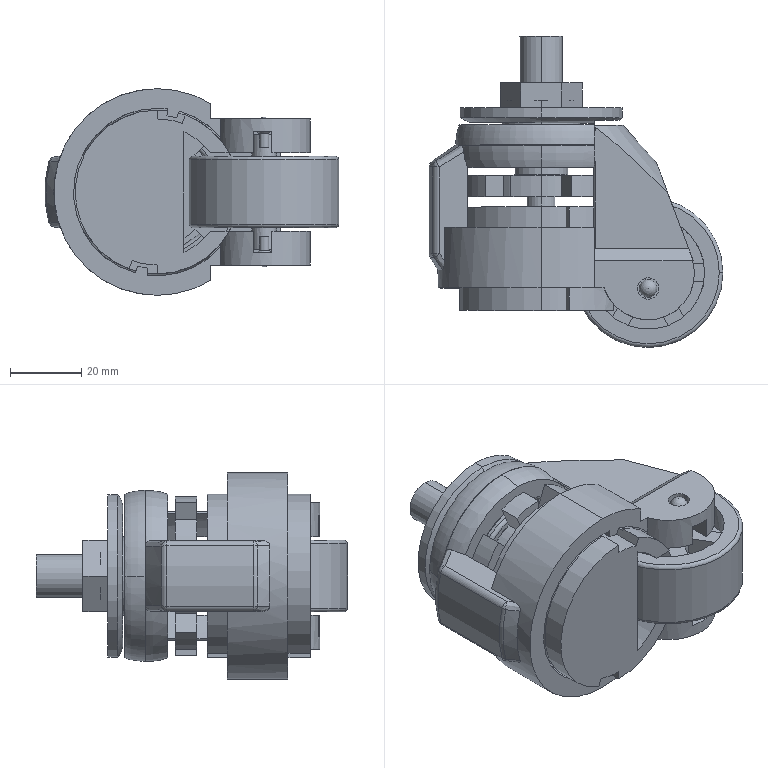Part | STEP file | Fuma wheel 60S01001 | 2 solids | 291 faces | box 82.6 x 87.32 x 58 mm | volume 125258 mm3 | plane 156 | cylinder 96 | torus 16 | sphere 8 | other 6 | cone 5 | spline 4 | commonest cylinder face diameters 46 x9 30 x8 44.62 x8 7 x6 2.6 x4 6 x4